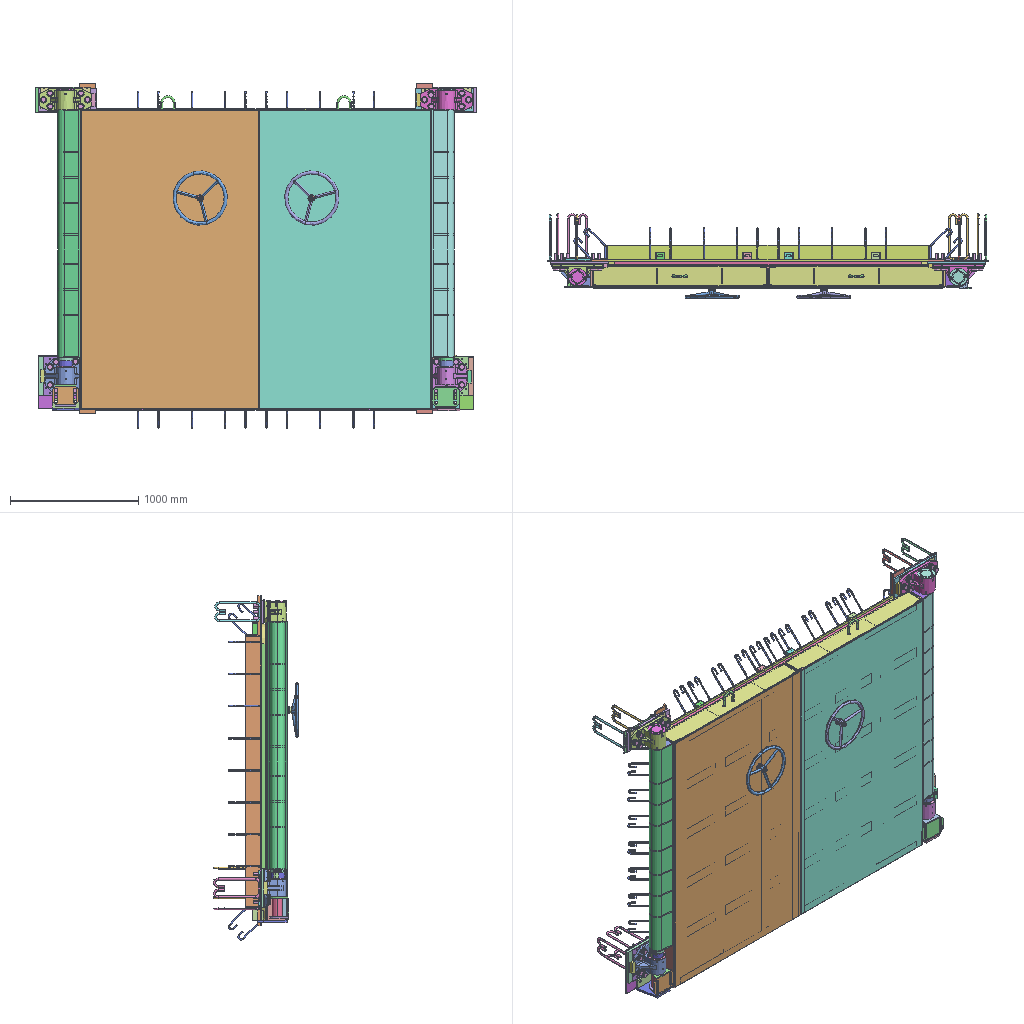Assembly | SolidWorks | 174 different items | 880 placed | box 3438 x 663 x 2684 mm
Parts list (item | name | quantity | parent item | size | volume | features):
1 | (subassembly) | x74 | - | 46.988 x 20.713 x 21.8 mm | 5348 mm3 | features MirrorCompFeat 1, ReferencePattern 1
2 | (subassembly) | x1 | in 3 | 425 x 574 x 434 mm | 5384557 mm3 | -
3 | (subassembly) | x1 | - | 2523 x 586.761 x 475 mm | 29684490 mm3 | features CompositeCurve 1
4 | (subassembly) | x1 | in 6 | 76 x 204 x 153 mm | 245569 mm3 | -
5 | (subassembly) | x1 | in 6 | 206.02 x 86.9 x 130 mm | 377637 mm3 | features CompositeCurve 2
6 | (subassembly) | x1 | - | - | 8515021 mm3 | features CompositeCurve 5
7 | (subassembly) | x1 | in 8 | 425 x 574 x 422 mm | 5384557 mm3 | features MirrorCompFeat 1, ReferencePattern 1
8 | (subassembly) | x1 | - | 2518 x 579 x 475 mm | 30927298 mm3 | features ReferencePattern 33, MirrorCompFeat 4, CompositeCurve 1, LocalCirPattern 1
9 | (subassembly) | x1 | - | 2740 x 211 x 2448 mm | 174205699 mm3 | features ReferencePattern 57, LocalLPattern 4, MirrorCompFeat 4
10 | (subassembly) | x1 | - | 3027 x 288.723 x 2684 mm | 36409651 mm3 | features ReferencePattern 81, MirrorCompFeat 5, LocalLPattern 4, CompositeCurve 1
11 | (subassembly) | x1 | in 13 | 76 x 129 x 157.154 mm | 245568 mm3 | -
12 | (subassembly) | x1 | in 13 | 206.02 x 86.9 x 130 mm | 377637 mm3 | features ReferencePattern 7, CompositeCurve 2, LocalLPattern 1, MirrorCompFeat 1
13 | (subassembly) | x1 | - | - | 8514992 mm3 | features ReferencePattern 98, CompositeCurve 5, LocalLPattern 4, MirrorCompFeat 2
14 | - | x1 | in 8 | 100 x 114 x 100 mm | 255348 mm3 | features Extrusion 1, HoleWzd 1, ICE 1
15 | - | x1 | in 3 | 140 x 2 x 140 mm | 17993 mm3 | features MirrorStock 1
16 | - | x1 | in 3 | 100 x 114 x 100 mm | 255348 mm3 | features MirrorStock 1
17 | - | x1 | in 3 | 56 x 44.676 x 56 mm | 61558 mm3 | features MirrorStock 1
18 | - | x1 | in 3 | 68 x 19 x 80 mm | 59636 mm3 | features MirrorStock 1
19 | - | x1 | in 3 | 68 x 7 x 80 mm | 21601 mm3 | features MirrorStock 1
20 | - | x1 | in 3 | 400 x 169 x 170 mm | 2936376 mm3 | features MirrorStock 1
21 | - | x1 | in 3 | 265 x 169 x 280 mm | 3133595 mm3 | features MirrorStock 1
22 | - | x1 | in 3 | 80 x 19 x 80 mm | 65180 mm3 | features MirrorStock 1
23 | - | x1 | in 3 | 166 x 140 x 210 mm | 892301 mm3 | features MirrorStock 1
24 | - | x1 | in 2 | 325 x 63 x 410 mm | 3290159 mm3 | features MirrorStock 1
25 | - | x1 | in 8 | 56 x 44.676 x 56 mm | 61558 mm3 | features Chamfer 1, HoleWzd 1, Revolution 1
26 | - | x1 | in 2 | 230 x 90 x 210 mm | 910703 mm3 | features MirrorStock 1
27 | - | x3 | in 2 | 156 x 364 x 16 mm | 207475 mm3 | features MirrorStock 1
28 | - | x2 | in 2 | 60 x 305 x 16 mm | 280636 mm3 | features MirrorStock 1
29 | - | x6 | in 3 | 94 x 1 x 265 mm | 13911 mm3 | features MirrorStock 1
30 | - | x1 | in 3 | 140 x 5 x 140 mm | 74707 mm3 | features MirrorStock 1
31 | - | x1 | in 3 | 140 x 2 x 140 mm | 29883 mm3 | features MirrorStock 1
32 | - | x1 | in 3 | 100 x 150 x 100 mm | 339747 mm3 | features MirrorStock 1
33 | - | x1 | in 3 | 65 x 330 x 80 mm | 1156605 mm3 | features MirrorStock 1
34 | - | x2 | in 9 | 95 x 16 x 95 mm | 9099 mm3 | features MirrorStock 1
35 | - | x1 | in 10 | 125 x 125 x 2570 mm | 5742663 mm3 | features MirrorStock 1
36 | - | x1 | in 8 | 68 x 19 x 80 mm | 59636 mm3 | features ICE 2, Extrusion 1, HoleWzd 1
37 | - | x2 | in 6 | 105 x 66 x 76 mm | 104524 mm3 | features MirrorStock 1
38 | - | x2 | in 6 | 113 x 40 x 255.904 mm | 148805 mm3 | features MirrorStock 1
39 | - | x6 | in 6 | 14 x 34.5 x 14 mm | 2794 mm3 | features MirrorStock 1
40 | - | x2 | in 6 | 275 x 22 x 20 mm | 44683 mm3 | features MirrorStock 1
41 | - | x4 | in 6 | 17 x 57 x 19.63 mm | 5343 mm3 | features MirrorStock 1
42 | - | x4 | in 6 | 50 x 3 x 50 mm | 3626 mm3 | features MirrorStock 1
43 | - | x4 | in 6 | 763 x 26 x 26 mm | 170096 mm3 | features MirrorStock 1
44 | - | x2 | in 6 | 50 x 130 x 50 mm | 135954 mm3 | features MirrorStock 1
45 | - | x4 | in 6 | 326 x 39.596 x 40 mm | 265934 mm3 | features MirrorStock 1
46 | - | x16 | in 6 | 40 x 2 x 160 mm | 9877 mm3 | features MirrorStock 1
47 | - | x1 | in 8 | 68 x 7 x 80 mm | 21601 mm3 | features Extrusion 1
48 | - | x4 | in 6 | 160 x 73 x 150 mm | 566023 mm3 | features MirrorStock 1
49 | - | x4 | in 6 | 18 x 40 x 18 mm | 6181 mm3 | features MirrorStock 1
50 | - | x2 | in 6 | 425 x 57.5 x 425 mm | 466638 mm3 | features MirrorStock 1
51 | - | x1 | in 6 | 40 x 372 x 40 mm | 221068 mm3 | features MirrorStock 1
52 | - | x1 | in 6 | 50 x 230 x 50 mm | 224751 mm3 | features MirrorStock 1
53 | - | x3 | in 6 | 50 x 4 x 50 mm | 4835 mm3 | features MirrorStock 1
54 | - | x2 | in 4, 6 | 76 x 76 x 24 mm | 54312 mm3 | features MirrorStock 1
55 | - | x3 | in 4 | 34 x 3 x 34 mm | 1251 mm3 | features MirrorStock 1
56 | - | x1 | in 4 | 34 x 73 x 34 mm | 37491 mm3 | features MirrorStock 1
57 | - | x1 | in 4 | 70 x 33 x 135 mm | 88171 mm3 | features MirrorStock 1
58 | - | x1 | in 8 | 400 x 169 x 170 mm | 2936377 mm3 | features Fillet 4, HoleWzd 3, ICE 2, Extrusion 1, MirrorPattern 1, Rib 1
59 | - | x1 | in 5 | 76 x 54 x 20 mm | 53995 mm3 | features MirrorStock 1
60 | - | x1 | in 5 | 137.5 x 29.697 x 30 mm | 38909 mm3 | features MirrorStock 1
61 | - | x1 | in 5 | 22.5 x 22.5 x 35 mm | 1475 mm3 | features MirrorStock 1
62 | - | x1 | in 5 | 90 x 64 x 130 mm | 252738 mm3 | features MirrorStock 1
63 | - | x2 | in 5 | 70 x 4 x 30 mm | 6843 mm3 | features MirrorStock 1
64 | - | x1 | in 5 | 20 x 20 x 6 mm | 1577 mm3 | features MirrorStock 1
65 | - | x1 | in 6 | 40 x 28 x 14 mm | 8141 mm3 | features MirrorStock 1
66 | - | x2 | in 6 | 40 x 100 x 40 mm | 63212 mm3 | features MirrorStock 1
67 | - | x1 | in 6 | 30 x 30 x 10 mm | 6265 mm3 | features MirrorStock 1
68 | - | x1 | in 6 | 38 x 888 x 38 mm | 315320 mm3 | features MirrorStock 1
69 | - | x1 | in 8 | 265 x 169 x 280 mm | 3133597 mm3 | features ICE 4, Fillet 2, HoleWzd 2, Rib 2, Chamfer 1, Extrusion 1
70 | - | x1 | in 9 | 95 x 16 x 95 mm | 9099 mm3 | features MirrorStock 1
71 | - | x1 | in 8 | 80 x 19 x 80 mm | 65180 mm3 | features Extrusion 1, HoleWzd 1, ICE 1, MirrorSolid 1, MoveCopyBody 1, Stock 1
72 | - | x1 | in 8 | 166 x 140 x 210 mm | 892301 mm3 | features ICE 3, Extrusion 1, MirrorSolid 1
73 | - | x1 | in 7 | 325 x 63 x 410 mm | 3290159 mm3 | features ICE 4, Extrusion 1, HoleWzd 1
74 | - | x1 | in 7 | 230 x 90 x 210 mm | 910703 mm3 | features Extrusion 1, HoleWzd 1, ICE 1
75 | - | x6 | in 8 | 100 x 1 x 165 mm | 11901 mm3 | features Extrusion 1, ICE 1
76 | - | x3 | in 7 | 156 x 364 x 16 mm | 207475 mm3 | features Sweep 1
77 | - | x2 | in 7 | 60 x 305 x 16 mm | 280636 mm3 | features Extrusion 1
78 | - | x6 | in 8 | 94 x 2 x 265 mm | 27822 mm3 | features Extrusion 1
79 | - | x1 | - | 160 x 5 x 140 mm | 84974 mm3 | features Extrusion 1
80 | - | x1 | in 8 | 140 x 5 x 140 mm | 74707 mm3 | features Extrusion 1, ICE 1
81 | - | x1 | in 8 | 140 x 2 x 140 mm | 29883 mm3 | features Extrusion 1, ICE 1
82 | - | x1 | in 8 | 100 x 150 x 100 mm | 339747 mm3 | features Extrusion 1, HoleWzd 1, ICE 1
83 | - | x1 | in 8 | 65 x 330 x 80 mm | 1156605 mm3 | features Chamfer 1, Extrusion 1, HoleWzd 1, ICE 1
84 | - | x1 | in 9 | 43 x 50 x 2090 mm | 1054401 mm3 | features Extrusion 1, ICE 1
85 | - | x2 | in 9 | 2200 x 24 x 4 mm | 178062 mm3 | features Chamfer 1, Extrusion 1, Fillet 1, ICE 1
86 | - | x1 | in 8 | 65 x 330 x 80 mm | 1109288 mm3 | features Chamfer 1, Extrusion 1, HoleWzd 1, ICE 1, RevCut 1
87 | - | x9 | in 9 | 35 x 50 x 8 mm | 7000 mm3 | features Extrusion 1
88 | - | x8 | in 9 | 160 x 24 x 170 mm | 630633 mm3 | features Extrusion 1, HoleWzd 1
89 | - | x4 | in 9 | 90 x 24 x 120 mm | 253752 mm3 | features Extrusion 1, HoleWzd 1
90 | - | x2 | in 9 | 70 x 24 x 135 mm | 222714 mm3 | features Extrusion 1, HoleWzd 1
91 | - | x2 | in 9 | 70 x 24 x 130 mm | 214914 mm3 | features Extrusion 1, HoleWzd 1
92 | - | x4 | in 9 | 65 x 160 x 2340 mm | 4766991 mm3 | features Extrusion 1, HoleWzd 1
93 | - | x16 | in 9 | 88 x 160 x 493 mm | 848530 mm3 | features Chamfer 1, Extrusion 1, ICE 1
94 | - | x4 | in 9 | 88 x 160 x 2320 mm | 4382373 mm3 | features Chamfer 1, Extrusion 1, ICE 1
95 | - | x8 | in 9 | 88 x 160 x 345 mm | 560895 mm3 | features Chamfer 2, Extrusion 1, ICE 1
96 | - | x1 | in 9 | 2324 x 8 x 1335 mm | 24803330 mm3 | features Extrusion 1
97 | - | x1 | in 8 | 1995 x 150 x 175 mm | 11290061 mm3 | features ICE 6, LPattern 3, Extrusion 1, MirrorSolid 1
98 | - | x1 | in 9 | 2324 x 8 x 1380 mm | 25639970 mm3 | features Extrusion 1
99 | - | x2 | in 9 | 2324 x 8 x 1330 mm | 24688354 mm3 | features Extrusion 1
100 | - | x2 | in 9 | 173 x 160 x 1348 mm | 2718229 mm3 | features Chamfer 2, ICE 2, Extrusion 1, HoleWzd 1, MirrorSolid 1, MoveCopyBody 1, Stock 1, Sweep 1
101 | - | x2 | in 9 | 65 x 160 x 1348 mm | 2648614 mm3 | features Extrusion 1, ICE 1
102 | - | x1 | - | 173 x 160 x 1098 mm | 2436946 mm3 | features Extrusion 1, HoleWzd 1, ICE 1, MirrorSolid 1, MoveCopyBody 1, Stock 1, Sweep 1
103 | - | x1 | in 9 | 95 x 16 x 95 mm | 9099 mm3 | features Extrusion 1, Fillet 1
104 | - | x6 | in 9 | 1185 x 24 x 4 mm | 74446 mm3 | features Extrusion 1, Fillet 1, ICE 1
105 | - | x1 | - | 125 x 125 x 1100 mm | 2472250 mm3 | features Extrusion 1, ICE 1
106 | - | x1 | in 10 | 125 x 125 x 2570 mm | 5742663 mm3 | features Extrusion 1, HoleWzd 1, ICE 1
107 | - | x10 | in 10 | 1180 x 30 x 15 mm | 531000 mm3 | features Extrusion 1
108 | - | x1 | in 8 | 118 x 25 x 116 mm | 19115 mm3 | features ExtruThin 1, ICE 1
109 | - | x4 | in 10 | 159 x 30 x 159 mm | 107089 mm3 | features Extrusion 1
110 | - | x4 | in 10 | 80 x 30 x 80 mm | 51247 mm3 | features Extrusion 1
111 | - | x1 | in 10 | 118 x 26 x 8 mm | 12272 mm3 | features Blend 1, BlendCut 1, ICE 1
112 | - | x4 | in 10 | 125 x 8 x 125 mm | 43919 mm3 | features Extrusion 1
113 | - | x1 | - | 30 x 4 x 26 mm | 2912 mm3 | features Extrusion 1
114 | - | x70 | in 10 | 80.953 x 280.953 x 12 mm | 42925 mm3 | features Sweep 1
115 | - | x2 | in 10 | 125 x 125 x 2500 mm | 6154176 mm3 | features ICE 2, BossThin 1, Extrusion 1, LPattern 1, MirrorSolid 1
116 | - | x1 | - | 2617 x 26 x 2217 mm | 9696679 mm3 | features Fillet 1, ICE 1, Sweep 1
117 | - | x2 | in 13 | 105 x 66 x 76 mm | 104524 mm3 | features Chamfer 1, Extrusion 1, ICE 1
118 | - | x2 | in 13 | 113 x 40 x 255.904 mm | 148805 mm3 | features ICE 2, Chamfer 1, Extrusion 1
119 | - | x1 | in 8 | 475 x 200 x 414 mm | 2531678 mm3 | features ICE 3, LPattern 2, Extrusion 1, HoleWzd 1, Sweep 1
120 | - | x6 | in 13 | 14 x 34.5 x 14 mm | 2794 mm3 | features ICE 2, Chamfer 1, Extrusion 1, Fillet 1
121 | - | x2 | in 13 | 275 x 22 x 20 mm | 44683 mm3 | features ICE 3, Extrusion 1, HoleWzd 1, MoveCopyBody 1, Stock 1
122 | - | x4 | in 13 | 17 x 57 x 19.63 mm | 5343 mm3 | features Chamfer 1, Extrusion 1, Fillet 1, Revolution 1
123 | - | x4 | in 13 | 50 x 3 x 50 mm | 3626 mm3 | features Extrusion 1
124 | - | x4 | in 13 | 763 x 26 x 26 mm | 170096 mm3 | features ICE 2, Extrusion 1, MirrorSolid 1
125 | - | x2 | in 13 | 50 x 130 x 50 mm | 135954 mm3 | features Fillet 2, Chamfer 1, Revolution 1
126 | - | x4 | in 13 | 326 x 39.596 x 40 mm | 265934 mm3 | features ICE 3, Chamfer 2, HoleWzd 1, Revolution 1
127 | - | x16 | in 13 | 40 x 2 x 160 mm | 9877 mm3 | features Extrusion 1
128 | - | x4 | in 13 | 160 x 73 x 150 mm | 566023 mm3 | features Chamfer 2, MirrorSolid 2, Extrusion 1, HoleWzd 1, ICE 1, Revolution 1
129 | - | x4 | in 13 | 18 x 40 x 18 mm | 6181 mm3 | features ICE 2, Chamfer 1, Extrusion 1, Fillet 1
130 | - | x1 | in 8 | 112 x 70 x 114 mm | 156072 mm3 | features ICE 3, Extrusion 1
131 | - | x2 | in 13 | 425 x 57.5 x 425 mm | 466626 mm3 | features Sweep 2, CirPattern 1, ICE 1, SweepCut 1
132 | - | x1 | in 13 | 40 x 372 x 40 mm | 221068 mm3 | features ICE 3, Chamfer 1, RefAxis 1, Revolution 1
133 | - | x1 | in 13 | 50 x 230 x 50 mm | 224751 mm3 | features Chamfer 1, Revolution 1
134 | - | x3 | in 13 | 50 x 4 x 50 mm | 4835 mm3 | features Extrusion 1
135 | - | x2 | in 11, 13 | 76 x 76 x 24 mm | 54312 mm3 | features Chamfer 2, Revolution 2, ICE 1
136 | - | x3 | in 11 | 34 x 2 x 34 mm | 834.093 mm3 | features Extrusion 1
137 | - | x1 | in 11 | 34 x 73 x 34 mm | 37491 mm3 | features Chamfer 2, Fillet 1, Revolution 1
138 | - | x1 | in 11 | 70 x 33 x 135 mm | 88171 mm3 | features Extrusion 1, ICE 1
139 | - | x1 | in 12 | 76 x 54 x 20 mm | 53995 mm3 | features ICE 2, Chamfer 1, Extrusion 1, HoleWzd 1
140 | - | x1 | in 12 | 137.5 x 29.697 x 30 mm | 38909 mm3 | features ICE 5, Chamfer 1, Extrusion 1, MirrorPattern 1
141 | - | x1 | in 8 | 140 x 50 x 140 mm | 66857 mm3 | features ICE 1, Revolution 1
142 | - | x1 | in 12 | 22.5 x 22.5 x 35 mm | 1475 mm3 | features Helix 1, ICE 1, RefAxis 1, Sweep 1
143 | - | x1 | in 12 | 90 x 64 x 130 mm | 252738 mm3 | features Extrusion 1, HoleWzd 1, Revolution 1
144 | - | x2 | in 12 | 70 x 4 x 30 mm | 6843 mm3 | features Extrusion 1
145 | - | x1 | in 12 | 20 x 20 x 6 mm | 1577 mm3 | features Extrusion 1, Fillet 1
146 | - | x1 | in 13 | 40 x 28 x 14 mm | 8141 mm3 | features Chamfer 1, Extrusion 1, Fillet 1, ICE 1
147 | - | x2 | in 13 | 40 x 100 x 40 mm | 63212 mm3 | features Extrusion 1, ICE 1
148 | - | x1 | in 13 | 30 x 30 x 10 mm | 6265 mm3 | features Chamfer 1, Extrusion 1, Fillet 1
149 | - | x1 | in 13 | 38 x 888 x 38 mm | 315320 mm3 | features ICE 2, Chamfer 1, Extrusion 1
150 | - | x121 | in 3, 4, 5, 6, 8, 11, 12, 13 | 56.4 x 18.475 x 16 mm | 5313 mm3 | features RevCut 3, Boss 1, Chamfer 1, Extrusion 1, Fillet 1, LPattern 1
151 | - | x22 | in 5, 6, 12, 13 | 27.6 x 5.8 x 2.9 mm | 176.57 mm3 | features Sweep 1
152 | - | x1 | in 8 | 140 x 2 x 140 mm | 17993 mm3 | features Extrusion 1, ICE 1
153 | - | x74 | in 1 | 30.965 x 15.09 x 21.8 mm | 3635 mm3 | features Boss 2, Chamfer 1, CompositeCurve 1, Extrusion 1, MirrorPattern 1
154 | - | x148 | in 1 | 31.676 x 19.79 x 2.171 mm | 856.64 mm3 | features Boss 2, DeleteBody 1, Extrusion 1, Scale 1
155 | - | x1 | in 3 | 100 x 1 x 40 mm | 4000 mm3 | features MirrorStock 1
156 | - | x6 | in 3 | 100 x 1 x 165 mm | 11901 mm3 | features MirrorStock 1
157 | - | x1 | in 3 | 65 x 330 x 80 mm | 1109288 mm3 | features MirrorStock 1
158 | - | x1 | in 3 | 1995 x 150 x 175 mm | 10047262 mm3 | features MirrorStock 1
159 | - | x1 | in 3 | 118 x 25 x 116 mm | 19115 mm3 | features MirrorStock 1
160 | - | x1 | in 3 | 475 x 200 x 414 mm | 2531678 mm3 | features MirrorStock 1
161 | - | x1 | in 3 | 112 x 70 x 114 mm | 156072 mm3 | features MirrorStock 1
162 | - | x1 | in 3 | 140 x 50 x 140 mm | 66857 mm3 | features MirrorStock 1
163 | - | x1 | in 8 | 100 x 1 x 40 mm | 4000 mm3 | features Extrusion 1
164 | clevis pins with head gb | x1 | - | - | - | -
165 | hex socket set screws with flat point gb | x1 | - | - | - | -
166 | hex thin nuts grades ab gb | x1 | - | - | - | -
167 | hex thin nuts-grades ab-chamfered gb | x1 | - | - | - | -
168 | hexagon nuts grade c gb | x1 | - | - | - | -
169 | hexagon socket set screws with dog point gb | x1 | - | - | - | -
170 | plain washers--product grade c gb | x1 | - | - | - | -
171 | plain washers-n series-grade a gb | x1 | - | - | - | -
172 | spring lock washers--normal type gb | x1 | - | - | - | -
173 | square set screws with long dog point gb | x1 | - | - | - | -
174 | thrust ball bearings gb | x1 | - | - | - | -
Mates (type | each side: item.copy, entity, surface, feature):
In the top assembly
Coincident | 92.1 face plane Boss-Extrude 1 | 97.1 face plane Boss-Extrude 1 | 2 times
Coincident | 106.1 face plane Boss-Extrude 1 | 119.1 face plane Boss-Extrude 1
Parallel | 35.1 face plane | 92.2 face plane Boss-Extrude 1
Width | 92.2 face plane Boss-Extrude 1 | 92.1 face plane Boss-Extrude 1 | 106.1 face plane Boss-Extrude 1 | 35.1 face plane
Coincident | 109.1 face plane Boss-Extrude 1 | 99.1 face plane Boss-Extrude 1
Width | 100.1 face plane Boss-Extrude 1 | 101.1 face plane Boss-Extrude 1 | 115.1 face plane Boss-Extrude 1 | 115.2 face plane Boss-Extrude 1
Concentric | 88.1 face cylinder M16 Tapped Hole 1 | 128.1 face cylinder Boss-Extrude 1 | 2 times
Coincident | 88.1 face plane Boss-Extrude 1 | 127.1 face plane Boss-Extrude 1
Concentric | 88.1 face cylinder M16 Tapped Hole 1 | 127.1 face cylinder Boss-Extrude 1 | 2 times
Concentric | 88.2 face cylinder M16 Tapped Hole 1 | 127.2 face cylinder Boss-Extrude 1 | 2 times
Concentric | 88.2 face cylinder M16 Tapped Hole 1 | 128.2 face cylinder Boss-Extrude 1
Concentric | 99.1 face cylinder Boss-Extrude 1 | 132.1 face cylinder Revolve 1
Coincident | 89.1 face plane Boss-Extrude 1 | 117.1 face plane Boss-Extrude 1
Concentric | 89.1 face cylinder M10 Tapped Hole 1 | 117.1 face cylinder Boss-Extrude 1 | 2 times
Coincident | 89.2 face plane Boss-Extrude 1 | 117.2 face plane Boss-Extrude 1
Concentric | 89.2 face cylinder M10 Tapped Hole 1 | 117.2 face cylinder Boss-Extrude 1 | 2 times
Parallel | 99.1 face plane Boss-Extrude 1 | 147.1 face plane Boss-Extrude 1
Concentric | 99.1 face cylinder Boss-Extrude 1 | 118.1 face cylinder Boss-Extrude 1
Coincident | 99.1 face plane Boss-Extrude 1 | 125.1 face plane Revolve 1
Coincident | 91.1 face plane Boss-Extrude 1 | 144.1 face plane Boss-Extrude 1
Concentric | 91.1 face cylinder M8 Tapped Hole 1 | 150.1 face cylinder BaseBody
Concentric | 91.1 face cylinder M8 Tapped Hole 1 | 150.2 face cylinder BaseBody
Coincident | 90.1 face plane Boss-Extrude 1 | 138.1 face plane Boss-Extrude 1
Coincident | 115.2 face plane Boss-Extrude 1 | 116.1 face plane Sweep 1
Symmetric | 107.1 face plane Boss-Extrude 1 | 107.2 face plane Boss-Extrude 1 | 116.1 plane
Symmetric | 107.3 face plane Boss-Extrude 1 | 107.4 face plane Boss-Extrude 1 | 116.1 plane
Concentric | 90.2 face cylinder M10 Tapped Hole 1 | 150.3 face cylinder BaseBody
Concentric | 90.2 face cylinder M10 Tapped Hole 1 | 150.4 face cylinder BaseBody
Concentric | 90.2 face cylinder M10 Tapped Hole 1 | 150.5 face cylinder BaseBody
In subassembly 1
Concentric | 154.1 face cylinder Extrude 4 | 153.1 face cylinder Extrude 3
Coincident | 153.1 face plane Mirror 1 | 154.1 face plane Extrude 4
In subassembly 3
Concentric | 20.1 face cylinder FMJ30-2 Upper绞座_Mirror | 32.1 face cylinder FMJ30-7衬套_Mirror | 2 times
Coincident | 160.1 face plane FMJ30-1 Upper绞Base_Mirror | 155.1 face plane FMJ30-10调整垫片_Mirror | 2 times
Coincident | 20.1 face plane FMJ30-2 Upper绞座_Mirror | 155.1 face plane FMJ30-10调整垫片_Mirror
Coincident | 20.1 face plane FMJ30-2 Upper绞座_Mirror | 31.1 face plane FMJ30-4密封垫_Mirror
Concentric | 20.1 face cylinder FMJ30-2 Upper绞座_Mirror | 31.1 face cylinder FMJ30-4密封垫_Mirror
Coincident | 30.1 face plane FMJ30-3盖Plate_Mirror | 31.1 face plane FMJ30-4密封垫_Mirror
Concentric | 30.1 face cylinder FMJ30-3盖Plate_Mirror | 31.1 face cylinder FMJ30-4密封垫_Mirror | 2 times
Concentric | 30.1 face cylinder FMJ30-3盖Plate_Mirror | 150.3 face cylinder BaseBody
Concentric | 20.1 face cylinder FMJ30-2 Upper绞座_Mirror | 150.6 face cylinder BaseBody
Concentric | 20.1 face cylinder FMJ30-2 Upper绞座_Mirror | 150.7 face cylinder BaseBody
Concentric | 20.1 face cylinder FMJ30-2 Upper绞座_Mirror | 150.8 face cylinder BaseBody
Concentric | 156.1 face cylinder FMJ30-14调整垫片_Mirror | 150.9 face cylinder BaseBody
Coincident | 156.1 face plane FMJ30-14调整垫片_Mirror | 156.2 face plane FMJ30-14调整垫片_Mirror | 3 times
Coincident | 156.2 face plane FMJ30-14调整垫片_Mirror | 156.3 face plane FMJ30-14调整垫片_Mirror | 3 times
Coincident | 20.1 face plane FMJ30-2 Upper绞座_Mirror | 156.3 face plane FMJ30-14调整垫片_Mirror
Concentric | 20.1 face cylinder FMJ30-2 Upper绞座_Mirror | 21.1 face cylinder FMJ30-30 Lower绞座_Mirror
Coincident | 20.1 face plane FMJ30-2 Upper绞座_Mirror | 21.1 face plane FMJ30-30 Lower绞座_Mirror
Concentric | 21.1 face cylinder FMJ30-30 Lower绞座_Mirror | 16.1 face cylinder FMJ30-23衬套_Mirror
Parallel | 21.1 face cylinder FMJ30-30 Lower绞座_Mirror | 16.1 face cylinder FMJ30-23衬套_Mirror
Coincident | 29.1 face plane FMJ30-34调整垫片_Mirror | 29.2 face plane FMJ30-34调整垫片_Mirror | 2 times
Coincident | 29.3 face plane FMJ30-34调整垫片_Mirror | 29.2 face plane FMJ30-34调整垫片_Mirror | 3 times
Coincident | 29.3 face plane FMJ30-34调整垫片_Mirror | 29.1 face plane FMJ30-34调整垫片_Mirror
Coincident | 21.1 face plane FMJ30-30 Lower绞座_Mirror | 29.4 face plane FMJ30-34调整垫片_Mirror
Concentric | 16.1 face cylinder FMJ30-23衬套_Mirror | 17.1 face cylinder FMJ30-24调心冠_Mirror
Concentric | 157.1 face sphere FMJ30-15 Lower绞轴_Mirror | 17.1 face sphere FMJ30-24调心冠_Mirror
Coincident | 21.1 face plane FMJ30-30 Lower绞座_Mirror | 16.1 face plane FMJ30-23衬套_Mirror
Concentric | 157.1 face cylinder FMJ30-15 Lower绞轴_Mirror | 18.1 face cylinder FMJ30-26承压Plate_Mirror
Parallel | 157.1 face plane FMJ30-15 Lower绞轴_Mirror | 18.1 face plane FMJ30-26承压Plate_Mirror
Coincident | 157.1 face plane FMJ30-15 Lower绞轴_Mirror | 18.1 face plane FMJ30-26承压Plate_Mirror
Coincident | 18.1 face plane FMJ30-26承压Plate_Mirror | 19.1 face plane FMJ30-28保持架_Mirror | 2 times
Concentric | 18.1 face cylinder FMJ30-26承压Plate_Mirror | 19.1 face cylinder FMJ30-28保持架_Mirror
Coincident | 21.1 face plane FMJ30-30 Lower绞座_Mirror | 15.1 face plane FMJ30-22密封垫_Mirror
Concentric | 158.1 face cylinder FMJ30-18钢管_Mirror | 162.1 face cylinder FMJ30-21挡圈_Mirror
Coincident | 162.1 face plane FMJ30-21挡圈_Mirror | 15.1 face plane FMJ30-22密封垫_Mirror
Concentric | 162.1 face cylinder FMJ30-21挡圈_Mirror | 15.1 face cylinder FMJ30-22密封垫_Mirror | 2 times
Concentric | 161.1 face cylinder FMJ30-20围封Plate_Mirror | 162.1 face cylinder FMJ30-21挡圈_Mirror
Coincident | 161.1 face plane FMJ30-20围封Plate_Mirror | 162.1 face plane FMJ30-21挡圈_Mirror
Concentric | 159.1 face cylinder FMJ30-19捆紧带_Mirror | 161.1 face cylinder FMJ30-20围封Plate_Mirror
Coincident | 19.1 face plane FMJ30-28保持架_Mirror | 22.1 face plane FMJ30-31 Pad_Mirror
Concentric | 21.1 face cylinder FMJ30-30 Lower绞座_Mirror | 22.1 face cylinder FMJ30-31 Pad_Mirror
Concentric | 21.1 edge | 22.1 face cylinder FMJ30-31 Pad_Mirror
Parallel | 19.1 face plane FMJ30-28保持架_Mirror | 22.1 face plane FMJ30-31 Pad_Mirror
Concentric | 21.1 face cylinder FMJ30-30 Lower绞座_Mirror | 162.1 face cylinder FMJ30-21挡圈_Mirror | 2 times
Concentric | 21.1 face cylinder FMJ30-30 Lower绞座_Mirror | 150.10 face cylinder BaseBody
Concentric | 21.1 face cylinder FMJ30-30 Lower绞座_Mirror | 150.11 face cylinder BaseBody
In subassembly 2
Parallel | 24.1 face plane FMJ30-33-1底Plate_Mirror | 27.1 plane
DistanceDim | 27.1 plane | 24.1 plane
In subassembly 6
Concentric | 45.1 face cylinder PFX30-21闭锁头_Mirror | 43.1 face cylinder PFX30-1连杆_Mirror
DistanceDim | 43.1 face plane PFX30-1连杆_Mirror | 45.1 face plane PFX30-21闭锁头_Mirror
Coincident | 46.1 face plane PFX30-23调整垫片_Mirror | 46.2 face plane PFX30-23调整垫片_Mirror | 2 times
Concentric | 49.1 face cylinder PFX30-28销轴_Mirror | 43.1 face cylinder PFX30-1连杆_Mirror
Coincident | 49.1 face plane PFX30-28销轴_Mirror | 43.1 face plane PFX30-1连杆_Mirror
Concentric | 49.1 face cylinder PFX30-28销轴_Mirror | 151.1 face cylinder Body
Coincident | 49.1 face cylinder PFX30-28销轴_Mirror | 151.1 vertex
Concentric | 39.1 face cylinder PFX30-14销轴_Mirror | 43.1 face cylinder PFX30-1连杆_Mirror
Coincident | 39.1 face plane PFX30-14销轴_Mirror | 43.1 face plane PFX30-1连杆_Mirror
Concentric | 39.1 face cylinder PFX30-14销轴_Mirror | 151.2 face cylinder Body
Coincident | 39.1 face cylinder PFX30-14销轴_Mirror | 151.2 vertex
Coincident | 46.3 face plane PFX30-23调整垫片_Mirror | 46.4 face plane PFX30-23调整垫片_Mirror | 2 times
Concentric | 45.2 face cylinder PFX30-21闭锁头_Mirror | 43.2 face cylinder PFX30-1连杆_Mirror
DistanceDim | 43.2 face plane PFX30-1连杆_Mirror | 45.2 face plane PFX30-21闭锁头_Mirror
Concentric | 151.3 face cylinder Body | 49.2 face cylinder PFX30-28销轴_Mirror
Coincident | 151.3 vertex | 49.2 face cylinder PFX30-28销轴_Mirror
Concentric | 49.2 face cylinder PFX30-28销轴_Mirror | 43.2 face cylinder PFX30-1连杆_Mirror
Coincident | 49.2 face plane PFX30-28销轴_Mirror | 43.2 face plane PFX30-1连杆_Mirror
Concentric | 39.2 face cylinder PFX30-14销轴_Mirror | 43.2 face cylinder PFX30-1连杆_Mirror
Coincident | 39.2 face plane PFX30-14销轴_Mirror | 43.2 face plane PFX30-1连杆_Mirror
Concentric | 39.2 face cylinder PFX30-14销轴_Mirror | 151.4 face cylinder Body
Coincident | 39.2 face cylinder PFX30-14销轴_Mirror | 151.4 vertex
Concentric | 43.2 face cylinder PFX30-1连杆_Mirror | 38.1 face cylinder PFX30-11摇臂_Mirror
DistanceDim | 43.2 face plane PFX30-1连杆_Mirror | 38.1 face plane PFX30-11摇臂_Mirror
Concentric | 50.1 face cylinder PFX30-32手轮_Mirror | 52.1 face cylinder PFX30-35轴套_Mirror
Coincident | 50.1 face plane PFX30-32手轮_Mirror | 51.1 face plane PFX30-34手轮轴_Mirror | 2 times
Concentric | 51.1 face cylinder PFX30-34手轮轴_Mirror | 52.1 face cylinder PFX30-35轴套_Mirror
Concentric | 51.1 face cylinder PFX30-34手轮轴_Mirror | 54.1 face cylinder PFX30-38链轮_Mirror
Concentric | 51.1 face cylinder PFX30-34手轮轴_Mirror | 53.1 face cylinder PFX30-36调整垫片_Mirror
Concentric | 51.1 face cylinder PFX30-34手轮轴_Mirror | 53.2 face cylinder PFX30-36调整垫片_Mirror
Coincident | 51.1 face plane PFX30-34手轮轴_Mirror | 53.2 face plane PFX30-36调整垫片_Mirror
Coincident | 51.1 face plane PFX30-34手轮轴_Mirror | 50.2 face plane PFX30-32手轮_Mirror | 2 times
Concentric | 52.1 face cylinder PFX30-35轴套_Mirror | 53.3 face cylinder PFX30-36调整垫片_Mirror
Coincident | 52.1 face plane PFX30-35轴套_Mirror | 53.3 face plane PFX30-36调整垫片_Mirror
Coincident | 52.1 face plane PFX30-35轴套_Mirror | 53.2 face plane PFX30-36调整垫片_Mirror
Concentric | 52.1 face cylinder PFX30-35轴套_Mirror | 50.2 face cylinder PFX30-32手轮_Mirror
Coincident | 53.3 face plane PFX30-36调整垫片_Mirror | 53.1 face plane PFX30-36调整垫片_Mirror
Concentric | 41.1 face cylinder PFX30-17 Bolt_Mirror | 66.1 face cylinder PFX30-5连杆座_Mirror
Coincident | 41.1 face plane PFX30-17 Bolt_Mirror | 66.1 face plane PFX30-5连杆座_Mirror
Concentric | 41.2 face cylinder PFX30-17 Bolt_Mirror | 66.1 face cylinder PFX30-5连杆座_Mirror
Coincident | 41.2 face plane PFX30-17 Bolt_Mirror | 66.1 face plane PFX30-5连杆座_Mirror
Concentric | 150.12 face cylinder BaseBody | 66.1 face cylinder PFX30-5连杆座_Mirror
Coincident | 150.12 face plane BaseHead | 66.1 face plane PFX30-5连杆座_Mirror
Concentric | 150.5 face cylinder BaseBody | 66.2 face cylinder PFX30-5连杆座_Mirror
Coincident | 150.5 face plane BaseHead | 66.2 face plane PFX30-5连杆座_Mirror
Concentric | 65.1 face cylinder PFX30-4齿条_Mirror | 66.1 face cylinder PFX30-5连杆座_Mirror
DistanceDim | 65.1 face plane PFX30-4齿条_Mirror | 66.1 face plane PFX30-5连杆座_Mirror
Parallel | 65.1 face plane PFX30-4齿条_Mirror | 66.1 face plane PFX30-5连杆座_Mirror
Concentric | 67.1 face cylinder PFX30-6滚轮_Mirror | 66.1 face cylinder PFX30-5连杆座_Mirror
DistanceDim | 66.1 face plane PFX30-5连杆座_Mirror | 67.1 face plane PFX30-6滚轮_Mirror
Concentric | 37.1 face cylinder PFX30-10导杆座_Mirror | 68.1 face cylinder PFX30-7导杆_Mirror
Concentric | 68.1 face cylinder PFX30-7导杆_Mirror | 66.1 face cylinder PFX30-5连杆座_Mirror | 3 times
Concentric | 68.1 face cylinder PFX30-7导杆_Mirror | 66.2 face cylinder PFX30-5连杆座_Mirror | 3 times
Concentric | 66.2 face cylinder PFX30-5连杆座_Mirror | 40.1 face cylinder PFX30-16连杆_Mirror
DistanceDim | 40.1 face plane PFX30-16连杆_Mirror | 66.2 face plane PFX30-5连杆座_Mirror
Concentric | 66.2 face cylinder PFX30-5连杆座_Mirror | 41.3 face cylinder PFX30-17 Bolt_Mirror
Coincident | 66.2 face plane PFX30-5连杆座_Mirror | 41.3 face plane PFX30-17 Bolt_Mirror
Concentric | 40.1 face cylinder PFX30-16连杆_Mirror | 38.1 face cylinder PFX30-11摇臂_Mirror
Concentric | 40.1 face cylinder PFX30-16连杆_Mirror | 39.3 face cylinder PFX30-14销轴_Mirror
Coincident | 40.1 face plane PFX30-16连杆_Mirror | 39.3 face plane PFX30-14销轴_Mirror
Concentric | 39.3 face cylinder PFX30-14销轴_Mirror | 151.5 face cylinder Body
Coincident | 39.3 face cylinder PFX30-14销轴_Mirror | 151.5 vertex
Concentric | 38.1 face cylinder PFX30-11摇臂_Mirror | 44.1 face cylinder PFX30-20摇臂轴_Mirror
Coincident | 38.1 face plane PFX30-11摇臂_Mirror | 42.1 edge
Concentric | 38.1 face cylinder PFX30-11摇臂_Mirror | 42.2 face cylinder PFX30-19 Washer_Mirror
Concentric | 38.1 face cylinder PFX30-11摇臂_Mirror | 43.1 face cylinder PFX30-1连杆_Mirror
DistanceDim | 43.1 face plane PFX30-1连杆_Mirror | 38.1 face plane PFX30-11摇臂_Mirror
Coincident | 44.1 face plane PFX30-20摇臂轴_Mirror | 42.2 face plane PFX30-19 Washer_Mirror
Concentric | 37.1 face cylinder PFX30-10导杆座_Mirror | 150.13 face cylinder BaseBody
Concentric | 37.2 face cylinder PFX30-10导杆座_Mirror | 150.14 face cylinder BaseBody
In subassembly 5
Coincident | 60.1 face plane PFX30-40-3推动杆_Mirror | 61.1 face plane PFX30-40-4 Spring_Mirror
Concentric | 60.1 face cylinder PFX30-40-3推动杆_Mirror | 59.1 edge
Concentric | 60.1 face cylinder PFX30-40-3推动杆_Mirror | 64.1 face cylinder PFX30-40-8滚轮_Mirror
DistanceDim | 60.1 face plane PFX30-40-3推动杆_Mirror | 64.1 face plane PFX30-40-8滚轮_Mirror
Concentric | 62.1 face cylinder PFX30-40-5 Fixed座_Mirror | 150.3 face cylinder BaseBody
Concentric | 150.4 face cylinder BaseBody | 63.1 face cylinder PFX30-40-6调整垫片_Mirror
Concentric | 150.5 face cylinder BaseBody | 63.1 face cylinder PFX30-40-6调整垫片_Mirror
In subassembly 9
Coincident | 92.3 plane | 9.1 plane
Symmetric | 92.3 face plane Boss-Extrude 1 | 92.3 face plane Boss-Extrude 1 | 9.1 plane
DistanceDim | 92.3 face plane Boss-Extrude 1 | 9.1 plane
Coincident | 92.3 face plane Boss-Extrude 1 | 100.2 face plane Boss-Extrude 1 | 2 times
DistanceDim | 92.3 face plane Boss-Extrude 1 | 100.2 face plane Boss-Extrude 1
Coincident | 92.3 face plane Boss-Extrude 1 | 94.1 face plane Boss-Extrude 1
Coincident | 100.2 face plane Boss-Extrude 1 | 94.1 face plane Boss-Extrude 1
Coincident | 92.3 face plane Boss-Extrude 1 | 101.2 face plane Boss-Extrude 1 | 3 times
Coincident | 92.3 face plane Boss-Extrude 1 | 93.1 face plane Boss-Extrude 1
Coincident | 95.1 face plane Boss-Extrude 1 | 94.1 face plane Boss-Extrude 1
Coincident | 100.2 face plane Boss-Extrude 1 | 99.2 face plane Boss-Extrude 1
DistanceDim | 92.4 face plane Boss-Extrude 1 | 99.2 face plane Boss-Extrude 1
DistanceDim | 100.2 face plane Boss-Extrude 1 | 99.2 face plane Boss-Extrude 1
Coincident | 92.3 face plane Boss-Extrude 1 | 84.1 face plane Boss-Extrude 1
DistanceDim | 84.1 face plane Boss-Extrude 1 | 99.2 face plane Boss-Extrude 1
Coincident | 92.3 face plane Boss-Extrude 1 | 85.1 face plane Boss-Extrude 1
DistanceDim | 85.1 face plane Boss-Extrude 1 | 92.3 face plane Boss-Extrude 1
Width | 92.3 face plane Boss-Extrude 1 | 92.3 face plane Boss-Extrude 1 | 85.1 face plane Boss-Extrude 1 | 85.1 face plane Boss-Extrude 1
Width | 92.3 face plane Boss-Extrude 1 | 92.3 face plane Boss-Extrude 1 | 84.1 face plane Boss-Extrude 1 | 84.1 face plane Boss-Extrude 1
Coincident | 104.1 face plane Boss-Extrude 1 | 85.1 face plane Boss-Extrude 1
Coincident | 99.2 face plane Boss-Extrude 1 | 104.1 face plane Boss-Extrude 1
Coincident | 99.2 face plane Boss-Extrude 1 | 103.1 face plane Boss-Extrude 1
Coincident | 103.1 face plane Boss-Extrude 1 | 104.1 face plane Boss-Extrude 1
Coincident | 103.1 edge | 104.1 face plane Boss-Extrude 1
Coincident | 99.2 face plane Boss-Extrude 1 | 104.2 face plane Boss-Extrude 1
Coincident | 103.1 face plane Boss-Extrude 1 | 104.2 face plane Boss-Extrude 1
Coincident | 103.1 edge | 104.2 face plane Boss-Extrude 1
Coincident | 34.1 face plane | 104.2 face plane Boss-Extrude 1
Coincident | 99.2 face plane Boss-Extrude 1 | 88.3 face plane Boss-Extrude 1
DistanceDim | 88.3 plane | 101.2 face plane Boss-Extrude 1
DistanceDim | 88.3 plane | 9.1 plane
Coincident | 99.2 face plane Boss-Extrude 1 | 89.3 face plane Boss-Extrude 1
Coincident | 99.2 face plane Boss-Extrude 1 | 91.2 face plane Boss-Extrude 1
DistanceDim | 89.3 plane | 88.4 plane
DistanceDim | 89.3 face plane Boss-Extrude 1 | 88.5 plane
DistanceDim | 88.5 plane | 91.2 plane
Coincident | 100.2 face plane Boss-Extrude 1 | 96.1 face plane Boss-Extrude 1
Coincident | 99.2 face plane Boss-Extrude 1 | 96.1 face plane Boss-Extrude 1 | 2 times
Coincident | 92.5 face plane Boss-Extrude 1 | 98.1 face plane Boss-Extrude 1
Coincident | 99.3 face plane Boss-Extrude 1 | 98.1 face plane Boss-Extrude 1 | 2 times
Coincident | 84.1 face plane Boss-Extrude 1 | 87.1 face plane Boss-Extrude 1 | 2 times
Coincident | 99.2 face plane Boss-Extrude 1 | 87.1 face plane Boss-Extrude 1
Coincident | 99.2 face plane Boss-Extrude 1 | 90.3 face plane Boss-Extrude 1
DistanceDim | 90.3 face plane Boss-Extrude 1 | 99.2 face plane Boss-Extrude 1
DistanceDim | 88.5 face plane Boss-Extrude 1 | 90.3 face plane Boss-Extrude 1
Coincident | 92.3 face plane Boss-Extrude 1 | 95.1 face plane Boss-Extrude 1
Coincident | 94.1 face plane Boss-Extrude 1 | 95.1 face plane Cut-Extrude 1
Coincident | 93.1 face plane Boss-Extrude 1 | 95.1 face plane Boss-Extrude 1
Coincident | 93.1 face plane Boss-Extrude 1 | 92.4 face plane Boss-Extrude 1
Coincident | 94.1 face plane Boss-Extrude 1 | 94.2 face plane Boss-Extrude 1
Coincident | 93.1 face plane Boss-Extrude 1 | 94.2 face plane Boss-Extrude 1
Coincident | 100.2 face plane Boss-Extrude 1 | 94.2 face plane Cut-Extrude 1
DistanceDim | 100.2 face plane Boss-Extrude 1 | 95.1 face plane Boss-Extrude 1
Coincident | 94.2 face plane Boss-Extrude 1 | 93.2 face plane Boss-Extrude 1
Coincident | 93.1 face plane Boss-Extrude 1 | 93.2 face plane Boss-Extrude 1
Coincident | 94.2 face plane Boss-Extrude 1 | 93.2 edge
In subassembly 10
DistanceDim | 106.2 face plane Cut-Extrude 1 | 115.3 face plane Boss-Extrude 1
Coincident | 106.2 face plane Boss-Extrude 1 | 115.3 face plane Boss-Extrude 1 | 2 times
Coincident | 106.2 face plane Boss-Extrude 1 | 115.4 face plane Boss-Extrude 1 | 2 times
DistanceDim | 106.2 face plane Cut-Extrude 1 | 115.4 face plane Boss-Extrude 1
Coincident | 115.3 face plane Boss-Extrude 1 | 112.1 face plane Boss-Extrude 1 | 2 times
Coincident | 35.2 face plane | 112.1 face plane Boss-Extrude 1
Coincident | 35.2 face plane | 112.2 face plane Boss-Extrude 1 | 2 times
Coincident | 115.4 face plane Boss-Extrude 1 | 112.2 edge
Coincident | 115.3 face plane Boss-Extrude 1 | 110.1 face plane Boss-Extrude 1
Coincident | 110.1 face plane Boss-Extrude 1 | 109.2 face plane Boss-Extrude 1
Coincident | 110.1 face plane Boss-Extrude 1 | 107.5 face plane Boss-Extrude 1 | 2 times
Coincident | 110.1 edge | 107.5 face plane Boss-Extrude 1
DistanceDim | 115.3 plane | 107.5 face plane Boss-Extrude 1
Coincident | 110.1 face plane Boss-Extrude 1 | 107.6 face plane Boss-Extrude 1 | 2 times
Coincident | 110.1 edge | 107.6 face plane Boss-Extrude 1
Coincident | 109.2 face plane Boss-Extrude 1 | 107.7 face plane Boss-Extrude 1 | 2 times
Coincident | 109.2 edge | 107.7 face plane Boss-Extrude 1
Parallel | 107.6 face plane Boss-Extrude 1 | 107.7 face plane Boss-Extrude 1
Coincident | 109.2 face plane Boss-Extrude 1 | 107.8 face plane Boss-Extrude 1 | 2 times
Coincident | 109.2 edge | 107.8 face plane Boss-Extrude 1
Coincident | 107.6 plane | 107.7 plane
Coincident | 115.3 plane | 111.1 plane
Coincident | 111.1 plane | 107.6 plane
Tangent | 106.2 face plane Boss-Extrude 1 | 114.1 face cylinder Sweep 1
DistanceDim | 114.1 plane | 115.3 face plane Boss-Extrude 1
DistanceDim | 106.2 face plane Boss-Extrude 1 | 114.1 face plane Sweep 1
Coincident | 114.1 plane | 114.2 plane
DistanceDim | 106.2 face plane Boss-Extrude 1 | 114.2 face plane Sweep 1
Tangent | 106.2 face plane Boss-Extrude 1 | 114.2 face cylinder Sweep 1
Coincident | 114.3 plane | 114.4 plane
Tangent | 115.3 face plane Boss-Extrude 1 | 114.3 face cylinder Sweep 1
DistanceDim | 114.3 plane | 115.3 edge
DistanceDim | 115.3 face plane Boss-Extrude 1 | 114.3 face plane Sweep 1
DistanceDim | 115.3 face plane Boss-Extrude 1 | 114.4 face plane Sweep 1
Tangent | 115.3 face plane Boss-Extrude 1 | 114.4 face cylinder Sweep 1
Width | 107.6 face plane Boss-Extrude 1 | 107.9 face plane Boss-Extrude 1 | 35.2 face plane | 106.2 face plane Boss-Extrude 1
Width | 107.5 face plane Boss-Extrude 1 | 107.10 face plane Boss-Extrude 1 | 115.4 face plane Boss-Extrude 1 | 115.3 face plane Boss-Extrude 1
Coincident | 111.1 edge | 115.3 face plane Boss-Extrude 1
In subassembly 13
Concentric | 124.1 face cylinder Boss-Extrude 1 | 126.1 face cylinder Boss-Extrude 1
DistanceDim | 124.1 face plane Cut-Extrude 1 | 126.1 face plane Boss-Extrude 1
Concentric | 126.1 face cylinder Revolve 1 | 128.3 face cylinder Revolve 1
Coincident | 128.3 edge | 127.3 face plane Boss-Extrude 1
Coincident | 128.3 face plane Boss-Extrude 1 | 127.3 face plane Boss-Extrude 1
Concentric | 128.3 face cylinder Boss-Extrude 1 | 150.15 face cylinder BaseBody
Coincident | 127.4 face plane Boss-Extrude 1 | 127.3 face plane Boss-Extrude 1 | 2 times
Concentric | 124.1 face cylinder Boss-Extrude 1 | 129.1 face cylinder Boss-Extrude 2
Coincident | 124.1 face plane Boss-Extrude 1 | 129.1 face plane Boss-Extrude 1
Concentric | 129.1 face cylinder Cut-Extrude 2 | 151.6 face cylinder Body
Coincident | 129.1 face cylinder Boss-Extrude 2 | 151.6 vertex
Concentric | 124.1 face cylinder Mirror 1 | 120.1 face cylinder Boss-Extrude 2
Coincident | 124.1 face plane Mirror 1 | 120.1 face plane Boss-Extrude 1
Concentric | 120.1 face cylinder Cut-Extrude 2 | 151.7 face cylinder Body
Coincident | 120.1 face cylinder Boss-Extrude 2 | 151.7 vertex
Coincident | 127.5 face plane Boss-Extrude 1 | 127.6 face plane Boss-Extrude 1 | 2 times
Coincident | 128.4 edge | 127.6 face plane Boss-Extrude 1
Coincident | 128.4 face plane Boss-Extrude 1 | 127.6 face plane Boss-Extrude 1
Concentric | 128.4 face cylinder Boss-Extrude 1 | 150.16 face cylinder BaseBody
Concentric | 128.4 face cylinder Revolve 1 | 126.2 face cylinder Revolve 1
Concentric | 126.2 face cylinder Boss-Extrude 1 | 124.2 face cylinder Boss-Extrude 1
DistanceDim | 124.2 face plane Cut-Extrude 1 | 126.2 face plane Boss-Extrude 1
Concentric | 151.8 face cylinder Body | 129.2 face cylinder Cut-Extrude 2
Coincident | 151.8 vertex | 129.2 face cylinder Boss-Extrude 2
Concentric | 129.2 face cylinder Boss-Extrude 2 | 124.2 face cylinder Boss-Extrude 1
Coincident | 129.2 face plane Boss-Extrude 1 | 124.2 face plane Boss-Extrude 1
Concentric | 120.2 face cylinder Boss-Extrude 2 | 124.2 face cylinder Mirror 1
Coincident | 120.2 face plane Boss-Extrude 1 | 124.2 face plane Mirror 1
Concentric | 120.2 face cylinder Cut-Extrude 2 | 151.9 face cylinder Body
Coincident | 120.2 face cylinder Boss-Extrude 2 | 151.9 vertex
Concentric | 118.2 face cylinder Boss-Extrude 2 | 124.2 face cylinder Mirror 1
DistanceDim | 124.2 face plane Mirror 1 | 118.2 face plane Boss-Extrude 2
Coincident | 135.1 face plane Revolve 2 | 135.2 face plane Revolve 2
Concentric | 131.1 face cylinder Boss-Extrude 1 | 133.1 face cylinder Revolve 1
Coincident | 131.1 face plane Boss-Extrude 1 | 132.2 face plane Cut-Extrude 2
Coincident | 131.1 face plane Boss-Extrude 1 | 132.2 face plane Revolve 1
Concentric | 132.2 face cylinder Revolve 1 | 133.1 face cylinder Revolve 1
Concentric | 132.2 face cylinder Revolve 1 | 135.2 face cylinder Revolve 1
Coincident | 132.2 face plane Revolve 1 | 135.2 face plane Revolve 1
Concentric | 132.2 face cylinder Revolve 1 | 134.1 face cylinder Boss-Extrude 1
Concentric | 132.2 face cylinder Revolve 1 | 134.2 face cylinder Boss-Extrude 1
Coincident | 132.2 face plane Revolve 1 | 134.2 face plane Boss-Extrude 1
Coincident | 132.2 face plane Cut-Extrude 1 | 131.2 face plane Boss-Extrude 1
Coincident | 132.2 face plane Revolve 1 | 131.2 face plane Boss-Extrude 1
Concentric | 133.1 face cylinder Revolve 1 | 134.3 face cylinder Boss-Extrude 1
Coincident | 133.1 face plane Revolve 1 | 134.3 face plane Boss-Extrude 1
Coincident | 133.1 face plane Revolve 1 | 134.2 face plane Boss-Extrude 1
Concentric | 133.1 face cylinder Revolve 1 | 131.2 face cylinder Boss-Extrude 1
Coincident | 134.3 face plane Boss-Extrude 1 | 134.1 face plane Boss-Extrude 1
Concentric | 147.2 face cylinder Boss-Extrude 1 | 122.1 face cylinder Revolve 1
Coincident | 147.2 face plane Boss-Extrude 1 | 122.1 face plane Boss-Extrude 1
Concentric | 147.2 face cylinder Boss-Extrude 1 | 122.2 face cylinder Revolve 1
Coincident | 147.2 face plane Boss-Extrude 1 | 122.2 face plane Boss-Extrude 1
Concentric | 147.2 face cylinder Boss-Extrude 1 | 150.17 face cylinder BaseBody
Coincident | 147.2 face plane Boss-Extrude 1 | 150.17 face plane BaseHead
Concentric | 147.3 face cylinder Boss-Extrude 1 | 150.18 face cylinder BaseBody
Coincident | 147.3 face plane Boss-Extrude 1 | 150.18 face plane BaseHead
Concentric | 146.1 face cylinder Boss-Extrude 1 | 147.2 face cylinder Boss-Extrude 1
DistanceDim | 146.1 face plane Boss-Extrude 1 | 147.2 face plane Cut-Extrude 1
Parallel | 146.1 face plane Boss-Extrude 1 | 147.2 face plane Cut-Extrude 1
Concentric | 148.1 face cylinder Boss-Extrude 1 | 147.2 face cylinder Boss-Extrude 1
DistanceDim | 147.2 face plane Cut-Extrude 1 | 148.1 face plane Boss-Extrude 1
Concentric | 117.3 face cylinder Boss-Extrude 2 | 149.1 face cylinder Boss-Extrude 2
Concentric | 149.1 face cylinder Boss-Extrude 2 | 147.2 face cylinder Cut-Extrude 1
Concentric | 149.1 face cylinder Cut-Extrude 2 | 147.2 face cylinder Boss-Extrude 1 | 2 times
Concentric | 149.1 face cylinder Boss-Extrude 2 | 147.3 face cylinder Cut-Extrude 1
Concentric | 149.1 face cylinder Cut-Extrude 2 | 147.3 face cylinder Boss-Extrude 1 | 2 times
Concentric | 147.3 face cylinder Boss-Extrude 1 | 121.1 face cylinder Boss-Extrude 3
DistanceDim | 121.1 face plane Boss-Extrude 3 | 147.3 face plane Cut-Extrude 1
Concentric | 147.3 face cylinder Boss-Extrude 1 | 122.3 face cylinder Revolve 1
Coincident | 147.3 face plane Boss-Extrude 1 | 122.3 face plane Boss-Extrude 1
Concentric | 121.1 face cylinder Boss-Extrude 1 | 118.2 face cylinder Boss-Extrude 2
Concentric | 121.1 face cylinder Boss-Extrude 1 | 120.3 face cylinder Boss-Extrude 2
Coincident | 121.1 face plane Boss-Extrude 1 | 120.3 face plane Boss-Extrude 1
Concentric | 120.3 face cylinder Cut-Extrude 2 | 151.5 face cylinder Body
Coincident | 120.3 face cylinder Boss-Extrude 2 | 151.5 vertex
Concentric | 118.2 face cylinder Boss-Extrude 1 | 125.2 face cylinder Revolve 1
Coincident | 118.2 face plane Boss-Extrude 1 | 123.1 edge
Concentric | 118.2 face cylinder Boss-Extrude 1 | 123.2 face cylinder Boss-Extrude 1
Concentric | 124.1 face cylinder Mirror 1 | 118.2 face cylinder Boss-Extrude 2
DistanceDim | 124.1 face plane Mirror 1 | 118.2 face plane Boss-Extrude 2
Concentric | 123.1 face cylinder Boss-Extrude 1 | 125.2 face cylinder Revolve 1
Coincident | 125.2 face plane Revolve 1 | 123.2 face plane Boss-Extrude 1
Concentric | 117.3 face cylinder Boss-Extrude 1 | 150.13 face cylinder BaseBody
Concentric | 117.4 face cylinder Boss-Extrude 1 | 150.19 face cylinder BaseBody
In subassembly 11
Coincident | 138.2 face plane Boss-Extrude 1 | 137.1 face plane Revolve 1
Concentric | 138.2 face cylinder Boss-Extrude 1 | 137.1 face cylinder Revolve 1
Concentric | 137.1 face cylinder Revolve 1 | 136.1 face cylinder Boss-Extrude 1
Coincident | 137.1 face plane Revolve 1 | 136.1 face plane Boss-Extrude 1
Coincident | 136.1 face plane Boss-Extrude 1 | 136.2 face plane Boss-Extrude 1
Concentric | 137.1 face cylinder Revolve 1 | 136.2 face cylinder Boss-Extrude 1
Concentric | 137.1 face cylinder Revolve 1 | 135.2 face cylinder Revolve 1
Coincident | 135.2 face plane Revolve 1 | 136.2 face plane Boss-Extrude 1
Concentric | 137.1 face cylinder Revolve 1 | 136.3 face cylinder Boss-Extrude 1
Coincident | 135.2 face plane Revolve 1 | 136.3 face plane Boss-Extrude 1
In subassembly 12
Concentric | 143.1 face cylinder Revolve 1 | 140.1 face cylinder Boss-Extrude 2
Coincident | 140.1 face cylinder Boss-Extrude 3 | 142.1 axis
Coincident | 140.1 face plane Boss-Extrude 1 | 142.1 face plane Cut-Extrude 1
Concentric | 140.1 face cylinder Boss-Extrude 3 | 139.1 edge
Parallel | 143.1 face plane Boss-Extrude 1 | 139.1 face plane Boss-Extrude 1
Concentric | 140.1 face cylinder Boss-Extrude 4 | 145.1 face cylinder Boss-Extrude 1
DistanceDim | 140.1 face plane Boss-Extrude 4 | 145.1 face plane Boss-Extrude 1
Concentric | 143.1 face cylinder Boss-Extrude 1 | 150.3 face cylinder BaseBody
Coincident | 143.1 face plane Boss-Extrude 1 | 144.2 face plane Boss-Extrude 1
Concentric | 150.4 face cylinder BaseBody | 144.2 face cylinder Boss-Extrude 1
Concentric | 150.5 face cylinder BaseBody | 144.2 face cylinder Boss-Extrude 1
In subassembly 8
DistanceDim | 119.2 face plane Boss-Extrude 1 | 58.1 face plane Boss-Extrude 1
Concentric | 58.1 face cylinder Boss-Extrude 3 | 82.1 face cylinder Boss-Extrude 1
Concentric | 58.1 face cylinder M10 Tapped Hole 2 | 82.1 face cylinder Cut-Extrude 1
Coincident | 119.2 face plane Boss-Extrude 2 | 163.1 face plane Boss-Extrude 1 | 2 times
Coincident | 119.2 face plane Boss-Extrude 1 | 163.1 face plane Boss-Extrude 1
Coincident | 58.1 face plane Boss-Extrude 1 | 163.1 face plane Boss-Extrude 1
Concentric | 97.2 face cylinder Boss-Extrude 4 | 83.1 face cylinder Boss-Extrude 2
Coincident | 97.2 face plane Boss-Extrude 4 | 83.1 face plane Boss-Extrude 1
Concentric | 97.2 face cylinder Boss-Extrude 2 | 58.1 face cylinder Boss-Extrude 3
Coincident | 97.2 face plane Boss-Extrude 3 | 58.1 face plane Boss-Extrude 3
Coincident | 58.1 face plane Boss-Extrude 3 | 81.1 face plane Boss-Extrude 1
Concentric | 58.1 face cylinder Boss-Extrude 3 | 81.1 face cylinder Boss-Extrude 1
Coincident | 80.1 face plane Boss-Extrude 1 | 81.1 face plane Boss-Extrude 1
Concentric | 80.1 face cylinder Boss-Extrude 1 | 81.1 face cylinder Boss-Extrude 1
Concentric | 80.1 face cylinder Cut-Extrude 1 | 81.1 face cylinder Cut-Extrude 1
Concentric | 80.1 face cylinder Cut-Extrude 1 | 150.3 face cylinder BaseBody
Concentric | 58.1 face cylinder Boss-Extrude 1 | 150.8 face cylinder BaseBody
Concentric | 58.1 face cylinder Boss-Extrude 1 | 150.20 face cylinder BaseBody
Concentric | 58.1 face cylinder Boss-Extrude 1 | 150.10 face cylinder BaseBody
Coincident | 75.1 face plane Boss-Extrude 1 | 119.2 face plane Boss-Extrude 1
Concentric | 75.1 face cylinder Cut-Extrude 1 | 150.21 face cylinder BaseBody
Coincident | 75.1 face plane Boss-Extrude 1 | 75.2 face plane Boss-Extrude 1 | 3 times
Coincident | 75.2 face plane Boss-Extrude 1 | 75.3 face plane Boss-Extrude 1 | 3 times
Coincident | 58.1 face plane Boss-Extrude 1 | 75.3 face plane Boss-Extrude 1
Concentric | 97.2 face cylinder Cut-Extrude 5 | 83.1 face cylinder M10 Tapped Hole 1
Concentric | 97.2 face cylinder Boss-Extrude 4 | 86.1 face cylinder Boss-Extrude 2
Concentric | 97.2 face cylinder Cut-Extrude 5 | 86.1 face cylinder M10 Tapped Hole 1
Concentric | 58.1 face cylinder Boss-Extrude 3 | 69.1 face cylinder Boss-Extrude 3
Coincident | 58.1 face plane Boss-Extrude 1 | 69.1 face plane Boss-Extrude 1
Concentric | 69.1 face cylinder Boss-Extrude 3 | 14.1 face cylinder Boss-Extrude 1
Parallel | 69.1 face cylinder M10 Tapped Hole 2 | 14.1 face cylinder Cut-Extrude 1
Coincident | 73.1 face plane Boss-Extrude 1 | 78.1 face plane Boss-Extrude 1
Concentric | 73.1 face cylinder M20 Tapped Hole 1 | 78.1 face cylinder Boss-Extrude 1 | 2 times
Coincident | 78.2 face plane Boss-Extrude 1 | 78.3 face plane Boss-Extrude 1 | 2 times
Coincident | 78.1 face plane Boss-Extrude 1 | 78.3 face plane Boss-Extrude 1 | 3 times
Coincident | 78.1 face plane Boss-Extrude 1 | 78.2 face plane Boss-Extrude 1
Coincident | 69.1 face plane Boss-Extrude 1 | 78.4 face plane Boss-Extrude 1
Concentric | 69.1 face cylinder Boss-Extrude 1 | 73.1 face cylinder M20 Tapped Hole 1 | 2 times
Concentric | 14.1 face cylinder Boss-Extrude 1 | 25.1 face cylinder Revolve 1
Concentric | 86.1 face sphere Cut-Revolve 1 | 25.1 face sphere Revolve 1
Coincident | 69.1 face plane Boss-Extrude 3 | 14.1 face plane Boss-Extrude 1
Concentric | 86.1 face cylinder Boss-Extrude 1 | 36.1 face cylinder Boss-Extrude 1
Parallel | 86.1 face plane Boss-Extrude 1 | 36.1 face plane Boss-Extrude 1
Coincident | 86.1 face plane Boss-Extrude 1 | 36.1 face plane Boss-Extrude 1
Coincident | 36.1 face plane Boss-Extrude 1 | 47.1 face plane Boss-Extrude 1 | 2 times
Concentric | 36.1 face cylinder Boss-Extrude 1 | 47.1 face cylinder Boss-Extrude 1
Coincident | 69.1 face plane Boss-Extrude 3 | 152.1 face plane Boss-Extrude 1
Concentric | 97.2 face cylinder Boss-Extrude 4 | 141.1 face cylinder Revolve 1
Coincident | 141.1 face plane Revolve 1 | 152.1 face plane Boss-Extrude 1
Concentric | 141.1 face cylinder Cut-Extrude 1 | 152.1 face cylinder Cut-Extrude 1
Concentric | 130.1 face cylinder Boss-Extrude 2 | 141.1 face cylinder Revolve 1
Coincident | 130.1 face plane Boss-Extrude 2 | 141.1 face plane Revolve 1
Concentric | 108.1 face cylinder Extrude-薄壁1 | 130.1 face cylinder Boss-Extrude 2
Coincident | 97.2 face plane Mirror 1 | 108.1 face plane Extrude-薄壁1
Coincident | 47.1 face plane Boss-Extrude 1 | 71.1 face plane Boss-Extrude 1
Concentric | 69.1 face cylinder Cut-Extrude 1 | 71.1 face cylinder M10 Tapped Hole 1
Concentric | 69.1 edge | 71.1 face cylinder M10 Tapped Hole 1
Parallel | 47.1 face plane Boss-Extrude 1 | 71.1 face plane Boss-Extrude 1
Concentric | 69.1 face cylinder Boss-Extrude 3 | 141.1 face cylinder Revolve 1
Concentric | 141.1 face cylinder Revolve 1 | 152.1 face cylinder Boss-Extrude 1
Concentric | 69.1 face cylinder M10 Tapped Hole 1 | 141.1 face cylinder Cut-Extrude 1
Concentric | 97.2 face cylinder Boss-Extrude 4 | 72.1 face cylinder Boss-Extrude 3
Coincident | 69.1 face plane Boss-Extrude 3 | 72.1 face plane Mirror 1
Concentric | 69.1 face cylinder Boss-Extrude 1 | 150.22 face cylinder BaseBody
Concentric | 69.1 face cylinder Boss-Extrude 1 | 150.23 face cylinder BaseBody
Parallel | 97.2 face plane Boss-Extrude 1 | 119.2 face plane Boss-Extrude 1
Coincident | 97.2 face plane Mirror 1 | 130.1 face plane Boss-Extrude 1
Parallel | 74.1 face plane Boss-Extrude 2 | 72.1 face plane Boss-Extrude 1
In subassembly 7
Coincident | 73.2 face plane Boss-Extrude 2 | 77.1 face plane Boss-Extrude 1
Coincident | 73.2 face plane Boss-Extrude 3 | 77.1 face plane Boss-Extrude 1
Parallel | 73.2 face plane Boss-Extrude 2 | 76.1 plane
Tangent | 73.2 face plane Boss-Extrude 2 | 76.1 face cylinder Sweep 1
DistanceDim | 76.1 plane | 73.2 face plane Boss-Extrude 1
DistanceDim | 76.1 plane | 73.2 plane
DistanceDim | 77.1 plane | 73.2 plane
Tangent | 73.2 face plane Boss-Extrude 2 | 76.2 face cylinder Sweep 1
DistanceDim | 76.2 plane | 73.2 face plane Boss-Extrude 1
DistanceDim | 76.2 plane | 73.2 plane
Tangent | 73.2 face plane Boss-Extrude 2 | 76.3 face cylinder Sweep 1
Coincident | 73.2 plane | 76.3 plane
DistanceDim | 73.2 face plane Boss-Extrude 3 | 76.3 plane
Coincident | 73.2 face plane Boss-Extrude 2 | 74.2 face plane Boss-Extrude 2
Concentric | 73.2 face cylinder Cut-Extrude 1 | 74.2 face cylinder M20 Tapped Hole 1 | 2 times